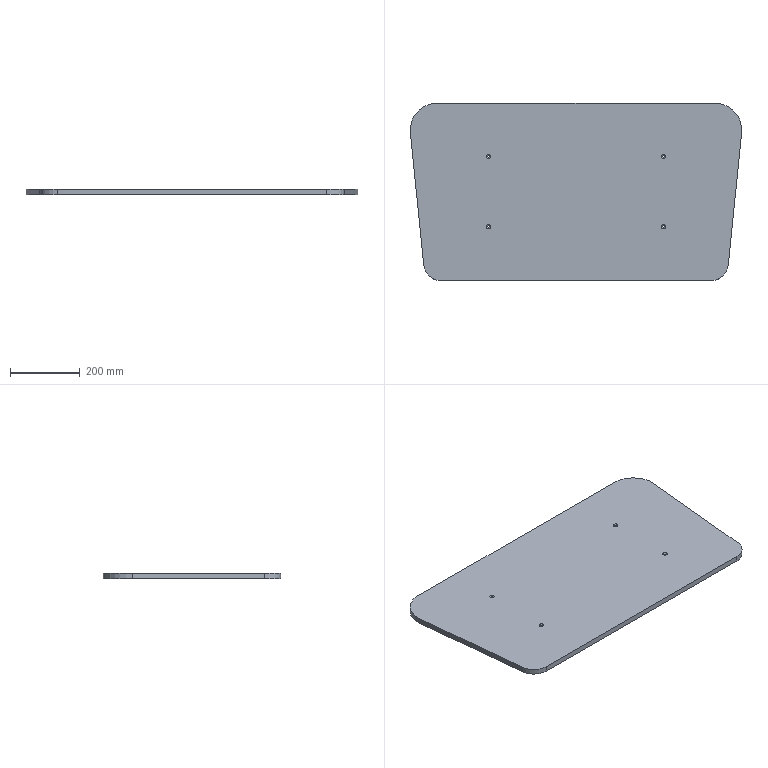Part | NX | features BREP 1 | 1 solid | 26 faces | box 949.2 x 508 x 15.875 mm | volume 7307811 mm3 | cylinder 12 | cone 8 | plane 6 | commonest cylinder face diameters 6.604 x8 101.6 x2 152.4 x2
STEP:
#1=CARTESIAN_POINT('',(-385.827,-508.,0.));
#2=VERTEX_POINT('',#1);
#3=CARTESIAN_POINT('',(385.827,-508.,0.));
#4=VERTEX_POINT('',#3);
#5=CARTESIAN_POINT('',(-385.827,-508.,0.));
#6=DIRECTION('',(1.,0.,0.));
#7=VECTOR('',#6,1000.);
#8=LINE('',#5,#7);
#9=EDGE_CURVE('',#2,#4,#8,.T.);
#10=ORIENTED_EDGE('',*,*,#9,.F.);
#11=CARTESIAN_POINT('',(-436.375,-462.255,0.));
#12=VERTEX_POINT('',#11);
#13=CARTESIAN_POINT('',(-385.827,-457.2,0.));
#14=DIRECTION('',(0.,0.,-1.));
#15=DIRECTION('',(0.,-1.,0.));
#16=AXIS2_PLACEMENT_3D('',#13,#14,#15);
#17=CIRCLE('',#16,50.8);
#18=EDGE_CURVE('',#2,#12,#17,.T.);
#19=ORIENTED_EDGE('',*,*,#18,.T.);
#20=CARTESIAN_POINT('',(-474.222,-83.782,0.));
#21=VERTEX_POINT('',#20);
#22=CARTESIAN_POINT('',(-474.222,-83.782,0.));
#23=DIRECTION('',(0.0995,-0.995,0.));
#24=VECTOR('',#23,1000.);
#25=LINE('',#22,#24);
#26=EDGE_CURVE('',#21,#12,#25,.T.);
#27=ORIENTED_EDGE('',*,*,#26,.F.);
#28=CARTESIAN_POINT('',(-398.4,0.,0.));
#29=VERTEX_POINT('',#28);
#30=CARTESIAN_POINT('',(-398.4,-76.2,0.));
#31=DIRECTION('',(0.,0.,-1.));
#32=DIRECTION('',(-0.995,-0.0995,0.));
#33=AXIS2_PLACEMENT_3D('',#30,#31,#32);
#34=CIRCLE('',#33,76.2);
#35=EDGE_CURVE('',#21,#29,#34,.T.);
#36=ORIENTED_EDGE('',*,*,#35,.T.);
#37=CARTESIAN_POINT('',(398.4,0.,0.));
#38=VERTEX_POINT('',#37);
#39=CARTESIAN_POINT('',(398.4,0.,0.));
#40=DIRECTION('',(-1.,0.,0.));
#41=VECTOR('',#40,1000.);
#42=LINE('',#39,#41);
#43=EDGE_CURVE('',#38,#29,#42,.T.);
#44=ORIENTED_EDGE('',*,*,#43,.F.);
#45=CARTESIAN_POINT('',(474.222,-83.782,0.));
#46=VERTEX_POINT('',#45);
#47=CARTESIAN_POINT('',(398.4,-76.2,0.));
#48=DIRECTION('',(0.,0.,-1.));
#49=DIRECTION('',(0.,1.,0.));
#50=AXIS2_PLACEMENT_3D('',#47,#48,#49);
#51=CIRCLE('',#50,76.2);
#52=EDGE_CURVE('',#38,#46,#51,.T.);
#53=ORIENTED_EDGE('',*,*,#52,.T.);
#54=CARTESIAN_POINT('',(436.375,-462.255,0.));
#55=VERTEX_POINT('',#54);
#56=CARTESIAN_POINT('',(436.375,-462.255,0.));
#57=DIRECTION('',(0.0995,0.995,0.));
#58=VECTOR('',#57,1000.);
#59=LINE('',#56,#58);
#60=EDGE_CURVE('',#55,#46,#59,.T.);
#61=ORIENTED_EDGE('',*,*,#60,.F.);
#62=CARTESIAN_POINT('',(385.827,-457.2,0.));
#63=DIRECTION('',(0.,0.,-1.));
#64=DIRECTION('',(0.995,-0.0995,0.));
#65=AXIS2_PLACEMENT_3D('',#62,#63,#64);
#66=CIRCLE('',#65,50.8);
#67=EDGE_CURVE('',#55,#4,#66,.T.);
#68=ORIENTED_EDGE('',*,*,#67,.T.);
#69=EDGE_LOOP('',(#10,#19,#27,#36,#44,#53,#61,#68));
#70=FACE_BOUND('',#69,.T.);
#71=CARTESIAN_POINT('',(-246.888,-353.06,0.));
#72=VERTEX_POINT('',#71);
#73=CARTESIAN_POINT('',(-253.492,-353.06,0.));
#74=VERTEX_POINT('',#73);
#75=CARTESIAN_POINT('',(-250.19,-353.06,0.));
#76=DIRECTION('',(0.,0.,1.));
#77=DIRECTION('',(1.,0.,0.));
#78=AXIS2_PLACEMENT_3D('',#75,#76,#77);
#79=CIRCLE('',#78,3.302);
#80=EDGE_CURVE('',#72,#74,#79,.T.);
#81=ORIENTED_EDGE('',*,*,#80,.T.);
#82=CARTESIAN_POINT('',(-250.19,-353.06,0.));
#83=DIRECTION('',(0.,0.,1.));
#84=DIRECTION('',(-1.,0.,0.));
#85=AXIS2_PLACEMENT_3D('',#82,#83,#84);
#86=CIRCLE('',#85,3.302);
#87=EDGE_CURVE('',#74,#72,#86,.T.);
#88=ORIENTED_EDGE('',*,*,#87,.T.);
#89=EDGE_LOOP('',(#81,#88));
#90=FACE_BOUND('',#89,.T.);
#91=CARTESIAN_POINT('',(253.492,-152.4,0.));
#92=VERTEX_POINT('',#91);
#93=CARTESIAN_POINT('',(246.888,-152.4,0.));
#94=VERTEX_POINT('',#93);
#95=CARTESIAN_POINT('',(250.19,-152.4,0.));
#96=DIRECTION('',(0.,0.,1.));
#97=DIRECTION('',(1.,0.,0.));
#98=AXIS2_PLACEMENT_3D('',#95,#96,#97);
#99=CIRCLE('',#98,3.302);
#100=EDGE_CURVE('',#92,#94,#99,.T.);
#101=ORIENTED_EDGE('',*,*,#100,.T.);
#102=CARTESIAN_POINT('',(250.19,-152.4,0.));
#103=DIRECTION('',(0.,0.,1.));
#104=DIRECTION('',(-1.,0.,0.));
#105=AXIS2_PLACEMENT_3D('',#102,#103,#104);
#106=CIRCLE('',#105,3.302);
#107=EDGE_CURVE('',#94,#92,#106,.T.);
#108=ORIENTED_EDGE('',*,*,#107,.T.);
#109=EDGE_LOOP('',(#101,#108));
#110=FACE_BOUND('',#109,.T.);
#111=CARTESIAN_POINT('',(253.492,-353.06,0.));
#112=VERTEX_POINT('',#111);
#113=CARTESIAN_POINT('',(246.888,-353.06,0.));
#114=VERTEX_POINT('',#113);
#115=CARTESIAN_POINT('',(250.19,-353.06,0.));
#116=DIRECTION('',(0.,0.,1.));
#117=DIRECTION('',(1.,0.,0.));
#118=AXIS2_PLACEMENT_3D('',#115,#116,#117);
#119=CIRCLE('',#118,3.302);
#120=EDGE_CURVE('',#112,#114,#119,.T.);
#121=ORIENTED_EDGE('',*,*,#120,.T.);
#122=CARTESIAN_POINT('',(250.19,-353.06,0.));
#123=DIRECTION('',(0.,0.,1.));
#124=DIRECTION('',(-1.,0.,0.));
#125=AXIS2_PLACEMENT_3D('',#122,#123,#124);
#126=CIRCLE('',#125,3.302);
#127=EDGE_CURVE('',#114,#112,#126,.T.);
#128=ORIENTED_EDGE('',*,*,#127,.T.);
#129=EDGE_LOOP('',(#121,#128));
#130=FACE_BOUND('',#129,.T.);
#131=CARTESIAN_POINT('',(-246.888,-152.4,0.));
#132=VERTEX_POINT('',#131);
#133=CARTESIAN_POINT('',(-253.492,-152.4,0.));
#134=VERTEX_POINT('',#133);
#135=CARTESIAN_POINT('',(-250.19,-152.4,0.));
#136=DIRECTION('',(0.,0.,1.));
#137=DIRECTION('',(1.,0.,0.));
#138=AXIS2_PLACEMENT_3D('',#135,#136,#137);
#139=CIRCLE('',#138,3.302);
#140=EDGE_CURVE('',#132,#134,#139,.T.);
#141=ORIENTED_EDGE('',*,*,#140,.T.);
#142=CARTESIAN_POINT('',(-250.19,-152.4,0.));
#143=DIRECTION('',(0.,0.,1.));
#144=DIRECTION('',(-1.,0.,0.));
#145=AXIS2_PLACEMENT_3D('',#142,#143,#144);
#146=CIRCLE('',#145,3.302);
#147=EDGE_CURVE('',#134,#132,#146,.T.);
#148=ORIENTED_EDGE('',*,*,#147,.T.);
#149=EDGE_LOOP('',(#141,#148));
#150=FACE_BOUND('',#149,.T.);
#151=CARTESIAN_POINT('',(0.,0.,0.));
#152=DIRECTION('',(0.,0.,1.));
#153=DIRECTION('',(1.,0.,0.));
#154=AXIS2_PLACEMENT_3D('',#151,#152,#153);
#155=PLANE('',#154);
#156=ADVANCED_FACE('',(#70,#90,#110,#130,#150),#155,.F.);
#157=CARTESIAN_POINT('',(246.888,-353.06,12.369));
#158=VERTEX_POINT('',#157);
#159=CARTESIAN_POINT('',(246.888,-353.06,0.));
#160=DIRECTION('',(0.,0.,1.));
#161=VECTOR('',#160,1000.);
#162=LINE('',#159,#161);
#163=EDGE_CURVE('',#114,#158,#162,.T.);
#164=ORIENTED_EDGE('',*,*,#163,.T.);
#165=CARTESIAN_POINT('',(253.492,-353.06,12.369));
#166=VERTEX_POINT('',#165);
#167=CARTESIAN_POINT('',(250.19,-353.06,12.369));
#168=DIRECTION('',(0.,0.,1.));
#169=DIRECTION('',(-1.,0.,0.));
#170=AXIS2_PLACEMENT_3D('',#167,#168,#169);
#171=CIRCLE('',#170,3.302);
#172=EDGE_CURVE('',#158,#166,#171,.T.);
#173=ORIENTED_EDGE('',*,*,#172,.T.);
#174=CARTESIAN_POINT('',(253.492,-353.06,0.));
#175=DIRECTION('',(0.,0.,1.));
#176=VECTOR('',#175,1000.);
#177=LINE('',#174,#176);
#178=EDGE_CURVE('',#112,#166,#177,.T.);
#179=ORIENTED_EDGE('',*,*,#178,.F.);
#180=ORIENTED_EDGE('',*,*,#127,.F.);
#181=EDGE_LOOP('',(#164,#173,#179,#180));
#182=FACE_BOUND('',#181,.T.);
#183=CARTESIAN_POINT('',(250.19,-353.06,-10.795));
#184=DIRECTION('',(0.,0.,1.));
#185=DIRECTION('',(-1.,0.,0.));
#186=AXIS2_PLACEMENT_3D('',#183,#184,#185);
#187=CYLINDRICAL_SURFACE('',#186,3.302);
#188=ADVANCED_FACE('',(#182),#187,.F.);
#189=ORIENTED_EDGE('',*,*,#178,.T.);
#190=CARTESIAN_POINT('',(250.19,-353.06,12.369));
#191=DIRECTION('',(0.,0.,-1.));
#192=DIRECTION('',(-1.,0.,0.));
#193=AXIS2_PLACEMENT_3D('',#190,#191,#192);
#194=CIRCLE('',#193,3.302);
#195=EDGE_CURVE('',#158,#166,#194,.T.);
#196=ORIENTED_EDGE('',*,*,#195,.F.);
#197=ORIENTED_EDGE('',*,*,#163,.F.);
#198=ORIENTED_EDGE('',*,*,#120,.F.);
#199=EDGE_LOOP('',(#189,#196,#197,#198));
#200=FACE_BOUND('',#199,.T.);
#201=CARTESIAN_POINT('',(250.19,-353.06,-10.795));
#202=DIRECTION('',(0.,0.,1.));
#203=DIRECTION('',(-1.,0.,0.));
#204=AXIS2_PLACEMENT_3D('',#201,#202,#203);
#205=CYLINDRICAL_SURFACE('',#204,3.302);
#206=ADVANCED_FACE('',(#200),#205,.F.);
#207=CARTESIAN_POINT('',(243.84,-353.06,15.875));
#208=VERTEX_POINT('',#207);
#209=CARTESIAN_POINT('',(246.888,-353.06,12.369));
#210=DIRECTION('',(-0.6561,0.,0.7547));
#211=VECTOR('',#210,1000.);
#212=LINE('',#209,#211);
#213=EDGE_CURVE('',#158,#208,#212,.T.);
#214=ORIENTED_EDGE('',*,*,#213,.F.);
#215=ORIENTED_EDGE('',*,*,#195,.T.);
#216=CARTESIAN_POINT('',(256.54,-353.06,15.875));
#217=VERTEX_POINT('',#216);
#218=CARTESIAN_POINT('',(253.492,-353.06,12.369));
#219=DIRECTION('',(0.6561,0.,0.7547));
#220=VECTOR('',#219,1000.);
#221=LINE('',#218,#220);
#222=EDGE_CURVE('',#166,#217,#221,.T.);
#223=ORIENTED_EDGE('',*,*,#222,.T.);
#224=CARTESIAN_POINT('',(250.19,-353.06,15.875));
#225=DIRECTION('',(0.,0.,1.));
#226=DIRECTION('',(1.,0.,0.));
#227=AXIS2_PLACEMENT_3D('',#224,#225,#226);
#228=CIRCLE('',#227,6.35);
#229=EDGE_CURVE('',#217,#208,#228,.T.);
#230=ORIENTED_EDGE('',*,*,#229,.T.);
#231=EDGE_LOOP('',(#214,#215,#223,#230));
#232=FACE_BOUND('',#231,.T.);
#233=CARTESIAN_POINT('',(250.19,-353.06,14.122));
#234=DIRECTION('',(0.,0.,1.));
#235=DIRECTION('',(-1.,0.,0.));
#236=AXIS2_PLACEMENT_3D('',#233,#234,#235);
#237=CONICAL_SURFACE('',#236,4.826,0.7156);
#238=ADVANCED_FACE('',(#232),#237,.F.);
#239=CARTESIAN_POINT('',(436.375,-462.255,15.875));
#240=VERTEX_POINT('',#239);
#241=CARTESIAN_POINT('',(474.222,-83.782,15.875));
#242=VERTEX_POINT('',#241);
#243=CARTESIAN_POINT('',(436.375,-462.255,15.875));
#244=DIRECTION('',(0.0995,0.995,0.));
#245=VECTOR('',#244,1000.);
#246=LINE('',#243,#245);
#247=EDGE_CURVE('',#240,#242,#246,.T.);
#248=ORIENTED_EDGE('',*,*,#247,.T.);
#249=CARTESIAN_POINT('',(398.4,0.,15.875));
#250=VERTEX_POINT('',#249);
#251=CARTESIAN_POINT('',(398.4,-76.2,15.875));
#252=DIRECTION('',(0.,0.,1.));
#253=DIRECTION('',(0.995,-0.0995,0.));
#254=AXIS2_PLACEMENT_3D('',#251,#252,#253);
#255=CIRCLE('',#254,76.2);
#256=EDGE_CURVE('',#242,#250,#255,.T.);
#257=ORIENTED_EDGE('',*,*,#256,.T.);
#258=CARTESIAN_POINT('',(-398.4,0.,15.875));
#259=VERTEX_POINT('',#258);
#260=CARTESIAN_POINT('',(398.4,0.,15.875));
#261=DIRECTION('',(-1.,0.,0.));
#262=VECTOR('',#261,1000.);
#263=LINE('',#260,#262);
#264=EDGE_CURVE('',#250,#259,#263,.T.);
#265=ORIENTED_EDGE('',*,*,#264,.T.);
#266=CARTESIAN_POINT('',(-474.222,-83.782,15.875));
#267=VERTEX_POINT('',#266);
#268=CARTESIAN_POINT('',(-398.4,-76.2,15.875));
#269=DIRECTION('',(0.,0.,1.));
#270=DIRECTION('',(0.,1.,0.));
#271=AXIS2_PLACEMENT_3D('',#268,#269,#270);
#272=CIRCLE('',#271,76.2);
#273=EDGE_CURVE('',#259,#267,#272,.T.);
#274=ORIENTED_EDGE('',*,*,#273,.T.);
#275=CARTESIAN_POINT('',(-436.375,-462.255,15.875));
#276=VERTEX_POINT('',#275);
#277=CARTESIAN_POINT('',(-474.222,-83.782,15.875));
#278=DIRECTION('',(0.0995,-0.995,0.));
#279=VECTOR('',#278,1000.);
#280=LINE('',#277,#279);
#281=EDGE_CURVE('',#267,#276,#280,.T.);
#282=ORIENTED_EDGE('',*,*,#281,.T.);
#283=CARTESIAN_POINT('',(-385.827,-508.,15.875));
#284=VERTEX_POINT('',#283);
#285=CARTESIAN_POINT('',(-385.827,-457.2,15.875));
#286=DIRECTION('',(0.,0.,1.));
#287=DIRECTION('',(-0.995,-0.0995,0.));
#288=AXIS2_PLACEMENT_3D('',#285,#286,#287);
#289=CIRCLE('',#288,50.8);
#290=EDGE_CURVE('',#276,#284,#289,.T.);
#291=ORIENTED_EDGE('',*,*,#290,.T.);
#292=CARTESIAN_POINT('',(385.827,-508.,15.875));
#293=VERTEX_POINT('',#292);
#294=CARTESIAN_POINT('',(-385.827,-508.,15.875));
#295=DIRECTION('',(1.,0.,0.));
#296=VECTOR('',#295,1000.);
#297=LINE('',#294,#296);
#298=EDGE_CURVE('',#284,#293,#297,.T.);
#299=ORIENTED_EDGE('',*,*,#298,.T.);
#300=CARTESIAN_POINT('',(385.827,-457.2,15.875));
#301=DIRECTION('',(0.,0.,1.));
#302=DIRECTION('',(0.,-1.,0.));
#303=AXIS2_PLACEMENT_3D('',#300,#301,#302);
#304=CIRCLE('',#303,50.8);
#305=EDGE_CURVE('',#293,#240,#304,.T.);
#306=ORIENTED_EDGE('',*,*,#305,.T.);
#307=EDGE_LOOP('',(#248,#257,#265,#274,#282,#291,#299,#306));
#308=FACE_BOUND('',#307,.T.);
#309=CARTESIAN_POINT('',(-243.84,-353.06,15.875));
#310=VERTEX_POINT('',#309);
#311=CARTESIAN_POINT('',(-256.54,-353.06,15.875));
#312=VERTEX_POINT('',#311);
#313=CARTESIAN_POINT('',(-250.19,-353.06,15.875));
#314=DIRECTION('',(0.,0.,1.));
#315=DIRECTION('',(1.,0.,0.));
#316=AXIS2_PLACEMENT_3D('',#313,#314,#315);
#317=CIRCLE('',#316,6.35);
#318=EDGE_CURVE('',#310,#312,#317,.T.);
#319=ORIENTED_EDGE('',*,*,#318,.F.);
#320=CARTESIAN_POINT('',(-250.19,-353.06,15.875));
#321=DIRECTION('',(0.,0.,1.));
#322=DIRECTION('',(-1.,0.,0.));
#323=AXIS2_PLACEMENT_3D('',#320,#321,#322);
#324=CIRCLE('',#323,6.35);
#325=EDGE_CURVE('',#312,#310,#324,.T.);
#326=ORIENTED_EDGE('',*,*,#325,.F.);
#327=EDGE_LOOP('',(#319,#326));
#328=FACE_BOUND('',#327,.T.);
#329=CARTESIAN_POINT('',(256.54,-152.4,15.875));
#330=VERTEX_POINT('',#329);
#331=CARTESIAN_POINT('',(243.84,-152.4,15.875));
#332=VERTEX_POINT('',#331);
#333=CARTESIAN_POINT('',(250.19,-152.4,15.875));
#334=DIRECTION('',(0.,0.,1.));
#335=DIRECTION('',(1.,0.,0.));
#336=AXIS2_PLACEMENT_3D('',#333,#334,#335);
#337=CIRCLE('',#336,6.35);
#338=EDGE_CURVE('',#330,#332,#337,.T.);
#339=ORIENTED_EDGE('',*,*,#338,.F.);
#340=CARTESIAN_POINT('',(250.19,-152.4,15.875));
#341=DIRECTION('',(0.,0.,1.));
#342=DIRECTION('',(-1.,0.,0.));
#343=AXIS2_PLACEMENT_3D('',#340,#341,#342);
#344=CIRCLE('',#343,6.35);
#345=EDGE_CURVE('',#332,#330,#344,.T.);
#346=ORIENTED_EDGE('',*,*,#345,.F.);
#347=EDGE_LOOP('',(#339,#346));
#348=FACE_BOUND('',#347,.T.);
#349=ORIENTED_EDGE('',*,*,#229,.F.);
#350=CARTESIAN_POINT('',(250.19,-353.06,15.875));
#351=DIRECTION('',(0.,0.,1.));
#352=DIRECTION('',(-1.,0.,0.));
#353=AXIS2_PLACEMENT_3D('',#350,#351,#352);
#354=CIRCLE('',#353,6.35);
#355=EDGE_CURVE('',#208,#217,#354,.T.);
#356=ORIENTED_EDGE('',*,*,#355,.F.);
#357=EDGE_LOOP('',(#349,#356));
#358=FACE_BOUND('',#357,.T.);
#359=CARTESIAN_POINT('',(-243.84,-152.4,15.875));
#360=VERTEX_POINT('',#359);
#361=CARTESIAN_POINT('',(-256.54,-152.4,15.875));
#362=VERTEX_POINT('',#361);
#363=CARTESIAN_POINT('',(-250.19,-152.4,15.875));
#364=DIRECTION('',(0.,0.,1.));
#365=DIRECTION('',(1.,0.,0.));
#366=AXIS2_PLACEMENT_3D('',#363,#364,#365);
#367=CIRCLE('',#366,6.35);
#368=EDGE_CURVE('',#360,#362,#367,.T.);
#369=ORIENTED_EDGE('',*,*,#368,.F.);
#370=CARTESIAN_POINT('',(-250.19,-152.4,15.875));
#371=DIRECTION('',(0.,0.,1.));
#372=DIRECTION('',(-1.,0.,0.));
#373=AXIS2_PLACEMENT_3D('',#370,#371,#372);
#374=CIRCLE('',#373,6.35);
#375=EDGE_CURVE('',#362,#360,#374,.T.);
#376=ORIENTED_EDGE('',*,*,#375,.F.);
#377=EDGE_LOOP('',(#369,#376));
#378=FACE_BOUND('',#377,.T.);
#379=CARTESIAN_POINT('',(0.,0.,15.875));
#380=DIRECTION('',(0.,0.,1.));
#381=DIRECTION('',(1.,0.,0.));
#382=AXIS2_PLACEMENT_3D('',#379,#380,#381);
#383=PLANE('',#382);
#384=ADVANCED_FACE('',(#308,#328,#348,#358,#378),#383,.T.);
#385=ORIENTED_EDGE('',*,*,#222,.F.);
#386=ORIENTED_EDGE('',*,*,#172,.F.);
#387=ORIENTED_EDGE('',*,*,#213,.T.);
#388=ORIENTED_EDGE('',*,*,#355,.T.);
#389=EDGE_LOOP('',(#385,#386,#387,#388));
#390=FACE_BOUND('',#389,.T.);
#391=CARTESIAN_POINT('',(250.19,-353.06,14.122));
#392=DIRECTION('',(0.,0.,1.));
#393=DIRECTION('',(-1.,0.,0.));
#394=AXIS2_PLACEMENT_3D('',#391,#392,#393);
#395=CONICAL_SURFACE('',#394,4.826,0.7156);
#396=ADVANCED_FACE('',(#390),#395,.F.);
#397=CARTESIAN_POINT('',(-246.888,-353.06,12.369));
#398=VERTEX_POINT('',#397);
#399=CARTESIAN_POINT('',(-246.888,-353.06,12.369));
#400=DIRECTION('',(0.6561,0.,0.7547));
#401=VECTOR('',#400,1000.);
#402=LINE('',#399,#401);
#403=EDGE_CURVE('',#310,#398,#402,.F.);
#404=ORIENTED_EDGE('',*,*,#403,.T.);
#405=CARTESIAN_POINT('',(-253.492,-353.06,12.369));
#406=VERTEX_POINT('',#405);
#407=CARTESIAN_POINT('',(-250.19,-353.06,12.369));
#408=DIRECTION('',(0.,0.,1.));
#409=DIRECTION('',(-1.,0.,0.));
#410=AXIS2_PLACEMENT_3D('',#407,#408,#409);
#411=CIRCLE('',#410,3.302);
#412=EDGE_CURVE('',#406,#398,#411,.T.);
#413=ORIENTED_EDGE('',*,*,#412,.F.);
#414=CARTESIAN_POINT('',(-253.492,-353.06,12.369));
#415=DIRECTION('',(-0.6561,0.,0.7547));
#416=VECTOR('',#415,1000.);
#417=LINE('',#414,#416);
#418=EDGE_CURVE('',#312,#406,#417,.F.);
#419=ORIENTED_EDGE('',*,*,#418,.F.);
#420=ORIENTED_EDGE('',*,*,#325,.T.);
#421=EDGE_LOOP('',(#404,#413,#419,#420));
#422=FACE_BOUND('',#421,.T.);
#423=CARTESIAN_POINT('',(-250.19,-353.06,14.122));
#424=DIRECTION('',(0.,0.,1.));
#425=DIRECTION('',(-1.,0.,0.));
#426=AXIS2_PLACEMENT_3D('',#423,#424,#425);
#427=CONICAL_SURFACE('',#426,4.826,0.7156);
#428=ADVANCED_FACE('',(#422),#427,.F.);
#429=ORIENTED_EDGE('',*,*,#418,.T.);
#430=CARTESIAN_POINT('',(-250.19,-353.06,12.369));
#431=DIRECTION('',(0.,0.,-1.));
#432=DIRECTION('',(-1.,0.,0.));
#433=AXIS2_PLACEMENT_3D('',#430,#431,#432);
#434=CIRCLE('',#433,3.302);
#435=EDGE_CURVE('',#406,#398,#434,.T.);
#436=ORIENTED_EDGE('',*,*,#435,.T.);
#437=ORIENTED_EDGE('',*,*,#403,.F.);
#438=ORIENTED_EDGE('',*,*,#318,.T.);
#439=EDGE_LOOP('',(#429,#436,#437,#438));
#440=FACE_BOUND('',#439,.T.);
#441=CARTESIAN_POINT('',(-250.19,-353.06,14.122));
#442=DIRECTION('',(0.,0.,1.));
#443=DIRECTION('',(-1.,0.,0.));
#444=AXIS2_PLACEMENT_3D('',#441,#442,#443);
#445=CONICAL_SURFACE('',#444,4.826,0.7156);
#446=ADVANCED_FACE('',(#440),#445,.F.);
#447=CARTESIAN_POINT('',(-246.888,-353.06,0.));
#448=DIRECTION('',(0.,0.,1.));
#449=VECTOR('',#448,1000.);
#450=LINE('',#447,#449);
#451=EDGE_CURVE('',#398,#72,#450,.F.);
#452=ORIENTED_EDGE('',*,*,#451,.F.);
#453=ORIENTED_EDGE('',*,*,#435,.F.);
#454=CARTESIAN_POINT('',(-253.492,-353.06,0.));
#455=DIRECTION('',(0.,0.,1.));
#456=VECTOR('',#455,1000.);
#457=LINE('',#454,#456);
#458=EDGE_CURVE('',#406,#74,#457,.F.);
#459=ORIENTED_EDGE('',*,*,#458,.T.);
#460=ORIENTED_EDGE('',*,*,#80,.F.);
#461=EDGE_LOOP('',(#452,#453,#459,#460));
#462=FACE_BOUND('',#461,.T.);
#463=CARTESIAN_POINT('',(-250.19,-353.06,-10.795));
#464=DIRECTION('',(0.,0.,1.));
#465=DIRECTION('',(-1.,0.,0.));
#466=AXIS2_PLACEMENT_3D('',#463,#464,#465);
#467=CYLINDRICAL_SURFACE('',#466,3.302);
#468=ADVANCED_FACE('',(#462),#467,.F.);
#469=ORIENTED_EDGE('',*,*,#458,.F.);
#470=ORIENTED_EDGE('',*,*,#412,.T.);
#471=ORIENTED_EDGE('',*,*,#451,.T.);
#472=ORIENTED_EDGE('',*,*,#87,.F.);
#473=EDGE_LOOP('',(#469,#470,#471,#472));
#474=FACE_BOUND('',#473,.T.);
#475=CARTESIAN_POINT('',(-250.19,-353.06,-10.795));
#476=DIRECTION('',(0.,0.,1.));
#477=DIRECTION('',(-1.,0.,0.));
#478=AXIS2_PLACEMENT_3D('',#475,#476,#477);
#479=CYLINDRICAL_SURFACE('',#478,3.302);
#480=ADVANCED_FACE('',(#474),#479,.F.);
#481=CARTESIAN_POINT('',(253.492,-152.4,12.369));
#482=VERTEX_POINT('',#481);
#483=CARTESIAN_POINT('',(253.492,-152.4,12.369));
#484=DIRECTION('',(0.6561,0.,0.7547));
#485=VECTOR('',#484,1000.);
#486=LINE('',#483,#485);
#487=EDGE_CURVE('',#330,#482,#486,.F.);
#488=ORIENTED_EDGE('',*,*,#487,.T.);
#489=CARTESIAN_POINT('',(246.888,-152.4,12.369));
#490=VERTEX_POINT('',#489);
#491=CARTESIAN_POINT('',(250.19,-152.4,12.369));
#492=DIRECTION('',(0.,0.,1.));
#493=DIRECTION('',(-1.,0.,0.));
#494=AXIS2_PLACEMENT_3D('',#491,#492,#493);
#495=CIRCLE('',#494,3.302);
#496=EDGE_CURVE('',#490,#482,#495,.T.);
#497=ORIENTED_EDGE('',*,*,#496,.F.);
#498=CARTESIAN_POINT('',(246.888,-152.4,12.369));
#499=DIRECTION('',(-0.6561,0.,0.7547));
#500=VECTOR('',#499,1000.);
#501=LINE('',#498,#500);
#502=EDGE_CURVE('',#332,#490,#501,.F.);
#503=ORIENTED_EDGE('',*,*,#502,.F.);
#504=ORIENTED_EDGE('',*,*,#345,.T.);
#505=EDGE_LOOP('',(#488,#497,#503,#504));
#506=FACE_BOUND('',#505,.T.);
#507=CARTESIAN_POINT('',(250.19,-152.4,14.122));
#508=DIRECTION('',(0.,0.,1.));
#509=DIRECTION('',(-1.,0.,0.));
#510=AXIS2_PLACEMENT_3D('',#507,#508,#509);
#511=CONICAL_SURFACE('',#510,4.826,0.7156);
#512=ADVANCED_FACE('',(#506),#511,.F.);
#513=ORIENTED_EDGE('',*,*,#502,.T.);
#514=CARTESIAN_POINT('',(250.19,-152.4,12.369));
#515=DIRECTION('',(0.,0.,-1.));
#516=DIRECTION('',(-1.,0.,0.));
#517=AXIS2_PLACEMENT_3D('',#514,#515,#516);
#518=CIRCLE('',#517,3.302);
#519=EDGE_CURVE('',#490,#482,#518,.T.);
#520=ORIENTED_EDGE('',*,*,#519,.T.);
#521=ORIENTED_EDGE('',*,*,#487,.F.);
#522=ORIENTED_EDGE('',*,*,#338,.T.);
#523=EDGE_LOOP('',(#513,#520,#521,#522));
#524=FACE_BOUND('',#523,.T.);
#525=CARTESIAN_POINT('',(250.19,-152.4,14.122));
#526=DIRECTION('',(0.,0.,1.));
#527=DIRECTION('',(-1.,0.,0.));
#528=AXIS2_PLACEMENT_3D('',#525,#526,#527);
#529=CONICAL_SURFACE('',#528,4.826,0.7156);
#530=ADVANCED_FACE('',(#524),#529,.F.);
#531=CARTESIAN_POINT('',(253.492,-152.4,0.));
#532=DIRECTION('',(0.,0.,1.));
#533=VECTOR('',#532,1000.);
#534=LINE('',#531,#533);
#535=EDGE_CURVE('',#482,#92,#534,.F.);
#536=ORIENTED_EDGE('',*,*,#535,.F.);
#537=ORIENTED_EDGE('',*,*,#519,.F.);
#538=CARTESIAN_POINT('',(246.888,-152.4,0.));
#539=DIRECTION('',(0.,0.,1.));
#540=VECTOR('',#539,1000.);
#541=LINE('',#538,#540);
#542=EDGE_CURVE('',#490,#94,#541,.F.);
#543=ORIENTED_EDGE('',*,*,#542,.T.);
#544=ORIENTED_EDGE('',*,*,#100,.F.);
#545=EDGE_LOOP('',(#536,#537,#543,#544));
#546=FACE_BOUND('',#545,.T.);
#547=CARTESIAN_POINT('',(250.19,-152.4,-10.795));
#548=DIRECTION('',(0.,0.,1.));
#549=DIRECTION('',(-1.,0.,0.));
#550=AXIS2_PLACEMENT_3D('',#547,#548,#549);
#551=CYLINDRICAL_SURFACE('',#550,3.302);
#552=ADVANCED_FACE('',(#546),#551,.F.);
#553=ORIENTED_EDGE('',*,*,#542,.F.);
#554=ORIENTED_EDGE('',*,*,#496,.T.);
#555=ORIENTED_EDGE('',*,*,#535,.T.);
#556=ORIENTED_EDGE('',*,*,#107,.F.);
#557=EDGE_LOOP('',(#553,#554,#555,#556));
#558=FACE_BOUND('',#557,.T.);
#559=CARTESIAN_POINT('',(250.19,-152.4,-10.795));
#560=DIRECTION('',(0.,0.,1.));
#561=DIRECTION('',(-1.,0.,0.));
#562=AXIS2_PLACEMENT_3D('',#559,#560,#561);
#563=CYLINDRICAL_SURFACE('',#562,3.302);
#564=ADVANCED_FACE('',(#558),#563,.F.);
#565=ORIENTED_EDGE('',*,*,#305,.F.);
#566=CARTESIAN_POINT('',(385.827,-508.,15.875));
#567=DIRECTION('',(0.,0.,-1.));
#568=VECTOR('',#567,1000.);
#569=LINE('',#566,#568);
#570=EDGE_CURVE('',#293,#4,#569,.T.);
#571=ORIENTED_EDGE('',*,*,#570,.T.);
#572=ORIENTED_EDGE('',*,*,#67,.F.);
#573=CARTESIAN_POINT('',(436.375,-462.255,15.875));
#574=DIRECTION('',(0.,0.,-1.));
#575=VECTOR('',#574,1000.);
#576=LINE('',#573,#575);
#577=EDGE_CURVE('',#240,#55,#576,.T.);
#578=ORIENTED_EDGE('',*,*,#577,.F.);
#579=EDGE_LOOP('',(#565,#571,#572,#578));
#580=FACE_BOUND('',#579,.T.);
#581=CARTESIAN_POINT('',(385.827,-457.2,17.62));
#582=DIRECTION('',(0.,0.,-1.));
#583=DIRECTION('',(0.995,-0.0995,0.));
#584=AXIS2_PLACEMENT_3D('',#581,#582,#583);
#585=CYLINDRICAL_SURFACE('',#584,50.8);
#586=ADVANCED_FACE('',(#580),#585,.T.);
#587=ORIENTED_EDGE('',*,*,#60,.T.);
#588=CARTESIAN_POINT('',(474.222,-83.782,15.875));
#589=DIRECTION('',(0.,0.,-1.));
#590=VECTOR('',#589,1000.);
#591=LINE('',#588,#590);
#592=EDGE_CURVE('',#242,#46,#591,.T.);
#593=ORIENTED_EDGE('',*,*,#592,.F.);
#594=ORIENTED_EDGE('',*,*,#247,.F.);
#595=ORIENTED_EDGE('',*,*,#577,.T.);
#596=EDGE_LOOP('',(#587,#593,#594,#595));
#597=FACE_BOUND('',#596,.T.);
#598=CARTESIAN_POINT('',(431.8,-508.,0.));
#599=DIRECTION('',(0.995,-0.0995,0.));
#600=DIRECTION('',(0.,0.,-1.));
#601=AXIS2_PLACEMENT_3D('',#598,#599,#600);
#602=PLANE('',#601);
#603=ADVANCED_FACE('',(#597),#602,.T.);
#604=ORIENTED_EDGE('',*,*,#256,.F.);
#605=ORIENTED_EDGE('',*,*,#592,.T.);
#606=ORIENTED_EDGE('',*,*,#52,.F.);
#607=CARTESIAN_POINT('',(398.4,0.,15.875));
#608=DIRECTION('',(0.,0.,-1.));
#609=VECTOR('',#608,1000.);
#610=LINE('',#607,#609);
#611=EDGE_CURVE('',#250,#38,#610,.T.);
#612=ORIENTED_EDGE('',*,*,#611,.F.);
#613=EDGE_LOOP('',(#604,#605,#606,#612));
#614=FACE_BOUND('',#613,.T.);
#615=CARTESIAN_POINT('',(398.4,-76.2,17.62));
#616=DIRECTION('',(0.,0.,-1.));
#617=DIRECTION('',(0.,1.,0.));
#618=AXIS2_PLACEMENT_3D('',#615,#616,#617);
#619=CYLINDRICAL_SURFACE('',#618,76.2);
#620=ADVANCED_FACE('',(#614),#619,.T.);
#621=ORIENTED_EDGE('',*,*,#43,.T.);
#622=CARTESIAN_POINT('',(-398.4,0.,15.875));
#623=DIRECTION('',(0.,0.,-1.));
#624=VECTOR('',#623,1000.);
#625=LINE('',#622,#624);
#626=EDGE_CURVE('',#259,#29,#625,.T.);
#627=ORIENTED_EDGE('',*,*,#626,.F.);
#628=ORIENTED_EDGE('',*,*,#264,.F.);
#629=ORIENTED_EDGE('',*,*,#611,.T.);
#630=EDGE_LOOP('',(#621,#627,#628,#629));
#631=FACE_BOUND('',#630,.T.);
#632=CARTESIAN_POINT('',(482.6,0.,0.));
#633=DIRECTION('',(0.,1.,0.));
#634=DIRECTION('',(1.,0.,0.));
#635=AXIS2_PLACEMENT_3D('',#632,#633,#634);
#636=PLANE('',#635);
#637=ADVANCED_FACE('',(#631),#636,.T.);
#638=ORIENTED_EDGE('',*,*,#273,.F.);
#639=ORIENTED_EDGE('',*,*,#626,.T.);
#640=ORIENTED_EDGE('',*,*,#35,.F.);
#641=CARTESIAN_POINT('',(-474.222,-83.782,15.875));
#642=DIRECTION('',(0.,0.,-1.));
#643=VECTOR('',#642,1000.);
#644=LINE('',#641,#643);
#645=EDGE_CURVE('',#267,#21,#644,.T.);
#646=ORIENTED_EDGE('',*,*,#645,.F.);
#647=EDGE_LOOP('',(#638,#639,#640,#646));
#648=FACE_BOUND('',#647,.T.);
#649=CARTESIAN_POINT('',(-398.4,-76.2,17.62));
#650=DIRECTION('',(0.,0.,-1.));
#651=DIRECTION('',(-0.995,-0.0995,0.));
#652=AXIS2_PLACEMENT_3D('',#649,#650,#651);
#653=CYLINDRICAL_SURFACE('',#652,76.2);
#654=ADVANCED_FACE('',(#648),#653,.T.);
#655=ORIENTED_EDGE('',*,*,#281,.F.);
#656=ORIENTED_EDGE('',*,*,#645,.T.);
#657=ORIENTED_EDGE('',*,*,#26,.T.);
#658=CARTESIAN_POINT('',(-436.375,-462.255,15.875));
#659=DIRECTION('',(0.,0.,-1.));
#660=VECTOR('',#659,1000.);
#661=LINE('',#658,#660);
#662=EDGE_CURVE('',#276,#12,#661,.T.);
#663=ORIENTED_EDGE('',*,*,#662,.F.);
#664=EDGE_LOOP('',(#655,#656,#657,#663));
#665=FACE_BOUND('',#664,.T.);
#666=CARTESIAN_POINT('',(-482.6,0.,0.));
#667=DIRECTION('',(-0.995,-0.0995,0.));
#668=DIRECTION('',(-0.0995,0.995,0.));
#669=AXIS2_PLACEMENT_3D('',#666,#667,#668);
#670=PLANE('',#669);
#671=ADVANCED_FACE('',(#665),#670,.T.);
#672=ORIENTED_EDGE('',*,*,#290,.F.);
#673=ORIENTED_EDGE('',*,*,#662,.T.);
#674=ORIENTED_EDGE('',*,*,#18,.F.);
#675=CARTESIAN_POINT('',(-385.827,-508.,15.875));
#676=DIRECTION('',(0.,0.,-1.));
#677=VECTOR('',#676,1000.);
#678=LINE('',#675,#677);
#679=EDGE_CURVE('',#284,#2,#678,.T.);
#680=ORIENTED_EDGE('',*,*,#679,.F.);
#681=EDGE_LOOP('',(#672,#673,#674,#680));
#682=FACE_BOUND('',#681,.T.);
#683=CARTESIAN_POINT('',(-385.827,-457.2,17.62));
#684=DIRECTION('',(0.,0.,-1.));
#685=DIRECTION('',(0.,-1.,0.));
#686=AXIS2_PLACEMENT_3D('',#683,#684,#685);
#687=CYLINDRICAL_SURFACE('',#686,50.8);
#688=ADVANCED_FACE('',(#682),#687,.T.);
#689=ORIENTED_EDGE('',*,*,#298,.F.);
#690=ORIENTED_EDGE('',*,*,#679,.T.);
#691=ORIENTED_EDGE('',*,*,#9,.T.);
#692=ORIENTED_EDGE('',*,*,#570,.F.);
#693=EDGE_LOOP('',(#689,#690,#691,#692));
#694=FACE_BOUND('',#693,.T.);
#695=CARTESIAN_POINT('',(-431.8,-508.,0.));
#696=DIRECTION('',(0.,-1.,0.));
#697=DIRECTION('',(0.,0.,-1.));
#698=AXIS2_PLACEMENT_3D('',#695,#696,#697);
#699=PLANE('',#698);
#700=ADVANCED_FACE('',(#694),#699,.T.);
#701=CARTESIAN_POINT('',(-246.888,-152.4,12.369));
#702=VERTEX_POINT('',#701);
#703=CARTESIAN_POINT('',(-246.888,-152.4,12.369));
#704=DIRECTION('',(0.6561,0.,0.7547));
#705=VECTOR('',#704,1000.);
#706=LINE('',#703,#705);
#707=EDGE_CURVE('',#360,#702,#706,.F.);
#708=ORIENTED_EDGE('',*,*,#707,.T.);
#709=CARTESIAN_POINT('',(-253.492,-152.4,12.369));
#710=VERTEX_POINT('',#709);
#711=CARTESIAN_POINT('',(-250.19,-152.4,12.369));
#712=DIRECTION('',(0.,0.,1.));
#713=DIRECTION('',(-1.,0.,0.));
#714=AXIS2_PLACEMENT_3D('',#711,#712,#713);
#715=CIRCLE('',#714,3.302);
#716=EDGE_CURVE('',#710,#702,#715,.T.);
#717=ORIENTED_EDGE('',*,*,#716,.F.);
#718=CARTESIAN_POINT('',(-253.492,-152.4,12.369));
#719=DIRECTION('',(-0.6561,0.,0.7547));
#720=VECTOR('',#719,1000.);
#721=LINE('',#718,#720);
#722=EDGE_CURVE('',#362,#710,#721,.F.);
#723=ORIENTED_EDGE('',*,*,#722,.F.);
#724=ORIENTED_EDGE('',*,*,#375,.T.);
#725=EDGE_LOOP('',(#708,#717,#723,#724));
#726=FACE_BOUND('',#725,.T.);
#727=CARTESIAN_POINT('',(-250.19,-152.4,14.122));
#728=DIRECTION('',(0.,0.,1.));
#729=DIRECTION('',(-1.,0.,0.));
#730=AXIS2_PLACEMENT_3D('',#727,#728,#729);
#731=CONICAL_SURFACE('',#730,4.826,0.7156);
#732=ADVANCED_FACE('',(#726),#731,.F.);
#733=ORIENTED_EDGE('',*,*,#722,.T.);
#734=CARTESIAN_POINT('',(-250.19,-152.4,12.369));
#735=DIRECTION('',(0.,0.,-1.));
#736=DIRECTION('',(-1.,0.,0.));
#737=AXIS2_PLACEMENT_3D('',#734,#735,#736);
#738=CIRCLE('',#737,3.302);
#739=EDGE_CURVE('',#710,#702,#738,.T.);
#740=ORIENTED_EDGE('',*,*,#739,.T.);
#741=ORIENTED_EDGE('',*,*,#707,.F.);
#742=ORIENTED_EDGE('',*,*,#368,.T.);
#743=EDGE_LOOP('',(#733,#740,#741,#742));
#744=FACE_BOUND('',#743,.T.);
#745=CARTESIAN_POINT('',(-250.19,-152.4,14.122));
#746=DIRECTION('',(0.,0.,1.));
#747=DIRECTION('',(-1.,0.,0.));
#748=AXIS2_PLACEMENT_3D('',#745,#746,#747);
#749=CONICAL_SURFACE('',#748,4.826,0.7156);
#750=ADVANCED_FACE('',(#744),#749,.F.);
#751=CARTESIAN_POINT('',(-246.888,-152.4,0.));
#752=DIRECTION('',(0.,0.,1.));
#753=VECTOR('',#752,1000.);
#754=LINE('',#751,#753);
#755=EDGE_CURVE('',#702,#132,#754,.F.);
#756=ORIENTED_EDGE('',*,*,#755,.F.);
#757=ORIENTED_EDGE('',*,*,#739,.F.);
#758=CARTESIAN_POINT('',(-253.492,-152.4,0.));
#759=DIRECTION('',(0.,0.,1.));
#760=VECTOR('',#759,1000.);
#761=LINE('',#758,#760);
#762=EDGE_CURVE('',#710,#134,#761,.F.);
#763=ORIENTED_EDGE('',*,*,#762,.T.);
#764=ORIENTED_EDGE('',*,*,#140,.F.);
#765=EDGE_LOOP('',(#756,#757,#763,#764));
#766=FACE_BOUND('',#765,.T.);
#767=CARTESIAN_POINT('',(-250.19,-152.4,-10.795));
#768=DIRECTION('',(0.,0.,1.));
#769=DIRECTION('',(-1.,0.,0.));
#770=AXIS2_PLACEMENT_3D('',#767,#768,#769);
#771=CYLINDRICAL_SURFACE('',#770,3.302);
#772=ADVANCED_FACE('',(#766),#771,.F.);
#773=ORIENTED_EDGE('',*,*,#762,.F.);
#774=ORIENTED_EDGE('',*,*,#716,.T.);
#775=ORIENTED_EDGE('',*,*,#755,.T.);
#776=ORIENTED_EDGE('',*,*,#147,.F.);
#777=EDGE_LOOP('',(#773,#774,#775,#776));
#778=FACE_BOUND('',#777,.T.);
#779=CARTESIAN_POINT('',(-250.19,-152.4,-10.795));
#780=DIRECTION('',(0.,0.,1.));
#781=DIRECTION('',(-1.,0.,0.));
#782=AXIS2_PLACEMENT_3D('',#779,#780,#781);
#783=CYLINDRICAL_SURFACE('',#782,3.302);
#784=ADVANCED_FACE('',(#778),#783,.F.);
#785=CLOSED_SHELL('',(#156,#188,#206,#238,#384,#396,#428,#446,#468,#480,#512,#530,#552,#564,#586,#603,#620,#637,#654,#671,#688,#700,#732,#750,#772,#784));
#786=MANIFOLD_SOLID_BREP('',#785);
#787=(LENGTH_UNIT()NAMED_UNIT(*)SI_UNIT(.MILLI.,.METRE.));
#788=UNCERTAINTY_MEASURE_WITH_UNIT(LENGTH_MEASURE(0.00001),#787,'','');
#789=(NAMED_UNIT(*)PLANE_ANGLE_UNIT()SI_UNIT($,.RADIAN.));
#790=(NAMED_UNIT(*)SI_UNIT($,.STERADIAN.)SOLID_ANGLE_UNIT());
#791=(GEOMETRIC_REPRESENTATION_CONTEXT(3)GLOBAL_UNCERTAINTY_ASSIGNED_CONTEXT((#788))GLOBAL_UNIT_ASSIGNED_CONTEXT((#787,#789,#790))REPRESENTATION_CONTEXT('',''));
#792=ADVANCED_BREP_SHAPE_REPRESENTATION('',(#786),#791);